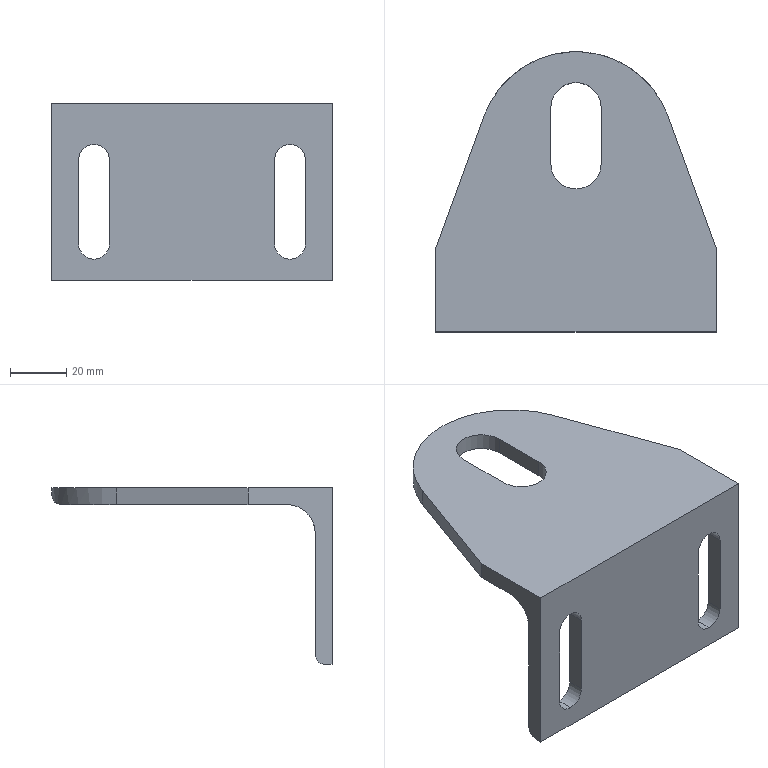Part | SolidWorks | features ICE 2, 3DProfileFeature 1, WeldMemberFeat 1, WeldmentFeature 1 | 1 solid | 29 faces | box 100 x 100 x 63 mm | volume 75285 mm3 | plane 16 | cylinder 13 | commonest cylinder face diameters 11 x6 6.667 x2 18 x2 70 x2 20 x1
STEP:
#1=CARTESIAN_POINT('',(85.,6.,-55.5));
#2=VERTEX_POINT('',#1);
#3=CARTESIAN_POINT('',(90.5,6.,-50.));
#4=VERTEX_POINT('',#3);
#5=CARTESIAN_POINT('',(85.,6.,-50.));
#6=DIRECTION('',(0.,-1.,0.));
#7=DIRECTION('',(0.,0.,-1.));
#8=AXIS2_PLACEMENT_3D('',#5,#6,#7);
#9=CIRCLE('',#8,5.5);
#10=EDGE_CURVE('',#2,#4,#9,.T.);
#11=ORIENTED_EDGE('',*,*,#10,.F.);
#12=CARTESIAN_POINT('',(85.,0.,-55.5));
#13=VERTEX_POINT('',#12);
#14=CARTESIAN_POINT('',(85.,15.,-55.5));
#15=DIRECTION('',(0.,-1.,0.));
#16=VECTOR('',#15,1000.);
#17=LINE('',#14,#16);
#18=EDGE_CURVE('',#2,#13,#17,.T.);
#19=ORIENTED_EDGE('',*,*,#18,.T.);
#20=CARTESIAN_POINT('',(90.5,0.,-50.));
#21=VERTEX_POINT('',#20);
#22=CARTESIAN_POINT('',(85.,0.,-50.));
#23=DIRECTION('',(0.,-1.,0.));
#24=DIRECTION('',(0.,0.,1.));
#25=AXIS2_PLACEMENT_3D('',#22,#23,#24);
#26=CIRCLE('',#25,5.5);
#27=EDGE_CURVE('',#13,#21,#26,.T.);
#28=ORIENTED_EDGE('',*,*,#27,.T.);
#29=CARTESIAN_POINT('',(90.5,15.,-50.));
#30=DIRECTION('',(0.,-1.,0.));
#31=VECTOR('',#30,1000.);
#32=LINE('',#29,#31);
#33=EDGE_CURVE('',#4,#21,#32,.T.);
#34=ORIENTED_EDGE('',*,*,#33,.F.);
#35=EDGE_LOOP('',(#11,#19,#28,#34));
#36=FACE_OUTER_BOUND('',#35,.T.);
#37=CARTESIAN_POINT('',(85.,15.,-50.));
#38=DIRECTION('',(0.,-1.,0.));
#39=DIRECTION('',(0.,0.,-1.));
#40=AXIS2_PLACEMENT_3D('',#37,#38,#39);
#41=CYLINDRICAL_SURFACE('',#40,5.5);
#42=ADVANCED_FACE('',(#36),#41,.F.);
#43=CARTESIAN_POINT('',(15.,6.,-55.5));
#44=VERTEX_POINT('',#43);
#45=CARTESIAN_POINT('',(20.5,6.,-50.));
#46=VERTEX_POINT('',#45);
#47=CARTESIAN_POINT('',(15.,6.,-50.));
#48=DIRECTION('',(0.,-1.,0.));
#49=DIRECTION('',(0.,0.,-1.));
#50=AXIS2_PLACEMENT_3D('',#47,#48,#49);
#51=CIRCLE('',#50,5.5);
#52=EDGE_CURVE('',#44,#46,#51,.T.);
#53=ORIENTED_EDGE('',*,*,#52,.F.);
#54=CARTESIAN_POINT('',(15.,0.,-55.5));
#55=VERTEX_POINT('',#54);
#56=CARTESIAN_POINT('',(15.,15.,-55.5));
#57=DIRECTION('',(0.,-1.,0.));
#58=VECTOR('',#57,1000.);
#59=LINE('',#56,#58);
#60=EDGE_CURVE('',#44,#55,#59,.T.);
#61=ORIENTED_EDGE('',*,*,#60,.T.);
#62=CARTESIAN_POINT('',(20.5,0.,-50.));
#63=VERTEX_POINT('',#62);
#64=CARTESIAN_POINT('',(15.,0.,-50.));
#65=DIRECTION('',(0.,-1.,0.));
#66=DIRECTION('',(0.,0.,-1.));
#67=AXIS2_PLACEMENT_3D('',#64,#65,#66);
#68=CIRCLE('',#67,5.5);
#69=EDGE_CURVE('',#55,#63,#68,.T.);
#70=ORIENTED_EDGE('',*,*,#69,.T.);
#71=CARTESIAN_POINT('',(20.5,15.,-50.));
#72=DIRECTION('',(0.,-1.,0.));
#73=VECTOR('',#72,1000.);
#74=LINE('',#71,#73);
#75=EDGE_CURVE('',#46,#63,#74,.T.);
#76=ORIENTED_EDGE('',*,*,#75,.F.);
#77=EDGE_LOOP('',(#53,#61,#70,#76));
#78=FACE_OUTER_BOUND('',#77,.T.);
#79=CARTESIAN_POINT('',(15.,15.,-50.));
#80=DIRECTION('',(0.,-1.,0.));
#81=DIRECTION('',(0.,0.,-1.));
#82=AXIS2_PLACEMENT_3D('',#79,#80,#81);
#83=CYLINDRICAL_SURFACE('',#82,5.5);
#84=ADVANCED_FACE('',(#78),#83,.F.);
#85=CARTESIAN_POINT('',(59.,60.,-6.));
#86=VERTEX_POINT('',#85);
#87=CARTESIAN_POINT('',(59.,80.,-6.));
#88=VERTEX_POINT('',#87);
#89=CARTESIAN_POINT('',(59.,96.667,-6.));
#90=DIRECTION('',(0.,1.,0.));
#91=VECTOR('',#90,1000.);
#92=LINE('',#89,#91);
#93=EDGE_CURVE('',#86,#88,#92,.T.);
#94=ORIENTED_EDGE('',*,*,#93,.T.);
#95=CARTESIAN_POINT('',(41.,80.,-6.));
#96=VERTEX_POINT('',#95);
#97=CARTESIAN_POINT('',(50.,80.,-6.));
#98=DIRECTION('',(0.,0.,1.));
#99=DIRECTION('',(0.,-1.,0.));
#100=AXIS2_PLACEMENT_3D('',#97,#98,#99);
#101=CIRCLE('',#100,9.);
#102=EDGE_CURVE('',#88,#96,#101,.T.);
#103=ORIENTED_EDGE('',*,*,#102,.T.);
#104=CARTESIAN_POINT('',(41.,60.,-6.));
#105=VERTEX_POINT('',#104);
#106=CARTESIAN_POINT('',(41.,96.667,-6.));
#107=DIRECTION('',(0.,-1.,0.));
#108=VECTOR('',#107,1000.);
#109=LINE('',#106,#108);
#110=EDGE_CURVE('',#96,#105,#109,.T.);
#111=ORIENTED_EDGE('',*,*,#110,.T.);
#112=CARTESIAN_POINT('',(50.,60.,-6.));
#113=DIRECTION('',(0.,0.,1.));
#114=DIRECTION('',(0.,-1.,0.));
#115=AXIS2_PLACEMENT_3D('',#112,#113,#114);
#116=CIRCLE('',#115,9.);
#117=EDGE_CURVE('',#105,#86,#116,.T.);
#118=ORIENTED_EDGE('',*,*,#117,.T.);
#119=EDGE_LOOP('',(#94,#103,#111,#118));
#120=FACE_BOUND('',#119,.T.);
#121=CARTESIAN_POINT('',(17.101,76.985,-6.));
#122=VERTEX_POINT('',#121);
#123=CARTESIAN_POINT('',(0.,30.,-6.));
#124=VERTEX_POINT('',#123);
#125=CARTESIAN_POINT('',(33.124,121.008,-6.));
#126=DIRECTION('',(-0.342,-0.9397,0.));
#127=VECTOR('',#126,1000.);
#128=LINE('',#125,#127);
#129=EDGE_CURVE('',#122,#124,#128,.T.);
#130=ORIENTED_EDGE('',*,*,#129,.F.);
#131=CARTESIAN_POINT('',(35.007,96.667,-6.));
#132=VERTEX_POINT('',#131);
#133=CARTESIAN_POINT('',(50.,65.041,-6.));
#134=DIRECTION('',(0.,0.,1.));
#135=DIRECTION('',(0.,-1.,0.));
#136=AXIS2_PLACEMENT_3D('',#133,#134,#135);
#137=CIRCLE('',#136,35.);
#138=EDGE_CURVE('',#132,#122,#137,.T.);
#139=ORIENTED_EDGE('',*,*,#138,.F.);
#140=CARTESIAN_POINT('',(64.993,96.667,-6.));
#141=VERTEX_POINT('',#140);
#142=CARTESIAN_POINT('',(100.,96.667,-6.));
#143=DIRECTION('',(-1.,0.,0.));
#144=VECTOR('',#143,1000.);
#145=LINE('',#142,#144);
#146=EDGE_CURVE('',#141,#132,#145,.T.);
#147=ORIENTED_EDGE('',*,*,#146,.F.);
#148=CARTESIAN_POINT('',(82.899,76.985,-6.));
#149=VERTEX_POINT('',#148);
#150=CARTESIAN_POINT('',(50.,65.041,-6.));
#151=DIRECTION('',(0.,0.,1.));
#152=DIRECTION('',(0.,-1.,0.));
#153=AXIS2_PLACEMENT_3D('',#150,#151,#152);
#154=CIRCLE('',#153,35.);
#155=EDGE_CURVE('',#149,#141,#154,.T.);
#156=ORIENTED_EDGE('',*,*,#155,.F.);
#157=CARTESIAN_POINT('',(100.,30.,-6.));
#158=VERTEX_POINT('',#157);
#159=CARTESIAN_POINT('',(78.574,88.868,-6.));
#160=DIRECTION('',(-0.342,0.9397,0.));
#161=VECTOR('',#160,1000.);
#162=LINE('',#159,#161);
#163=EDGE_CURVE('',#158,#149,#162,.T.);
#164=ORIENTED_EDGE('',*,*,#163,.F.);
#165=CARTESIAN_POINT('',(100.,16.,-6.));
#166=VERTEX_POINT('',#165);
#167=CARTESIAN_POINT('',(100.,96.667,-6.));
#168=DIRECTION('',(0.,1.,0.));
#169=VECTOR('',#168,1000.);
#170=LINE('',#167,#169);
#171=EDGE_CURVE('',#166,#158,#170,.T.);
#172=ORIENTED_EDGE('',*,*,#171,.F.);
#173=CARTESIAN_POINT('',(0.,16.,-6.));
#174=VERTEX_POINT('',#173);
#175=CARTESIAN_POINT('',(100.,16.,-6.));
#176=DIRECTION('',(-1.,0.,0.));
#177=VECTOR('',#176,1000.);
#178=LINE('',#175,#177);
#179=EDGE_CURVE('',#166,#174,#178,.T.);
#180=ORIENTED_EDGE('',*,*,#179,.T.);
#181=CARTESIAN_POINT('',(0.,96.667,-6.));
#182=DIRECTION('',(0.,1.,0.));
#183=VECTOR('',#182,1000.);
#184=LINE('',#181,#183);
#185=EDGE_CURVE('',#174,#124,#184,.T.);
#186=ORIENTED_EDGE('',*,*,#185,.T.);
#187=EDGE_LOOP('',(#130,#139,#147,#156,#164,#172,#180,#186));
#188=FACE_OUTER_BOUND('',#187,.T.);
#189=CARTESIAN_POINT('',(100.,96.667,-6.));
#190=DIRECTION('',(0.,0.,1.));
#191=DIRECTION('',(0.,-1.,0.));
#192=AXIS2_PLACEMENT_3D('',#189,#190,#191);
#193=PLANE('',#192);
#194=ADVANCED_FACE('',(#120,#188),#193,.F.);
#195=CARTESIAN_POINT('',(51.688,100.,-2.667));
#196=VERTEX_POINT('',#195);
#197=CARTESIAN_POINT('',(64.993,96.667,-6.));
#198=CARTESIAN_POINT('',(63.904,97.183,-6.));
#199=CARTESIAN_POINT('',(62.807,97.635,-5.885));
#200=CARTESIAN_POINT('',(61.142,98.225,-5.621));
#201=CARTESIAN_POINT('',(60.584,98.407,-5.517));
#202=CARTESIAN_POINT('',(59.462,98.743,-5.283));
#203=CARTESIAN_POINT('',(58.896,98.896,-5.152));
#204=CARTESIAN_POINT('',(57.196,99.313,-4.732));
#205=CARTESIAN_POINT('',(56.058,99.532,-4.414));
#206=CARTESIAN_POINT('',(54.353,99.774,-3.889));
#207=CARTESIAN_POINT('',(53.785,99.84,-3.707));
#208=CARTESIAN_POINT('',(52.939,99.918,-3.408));
#209=CARTESIAN_POINT('',(52.658,99.941,-3.304));
#210=CARTESIAN_POINT('',(52.246,99.969,-3.125));
#211=CARTESIAN_POINT('',(52.11,99.977,-3.062));
#212=CARTESIAN_POINT('',(51.916,99.988,-2.948));
#213=CARTESIAN_POINT('',(51.853,99.992,-2.907));
#214=CARTESIAN_POINT('',(51.769,99.996,-2.831));
#215=CARTESIAN_POINT('',(51.743,99.997,-2.804));
#216=CARTESIAN_POINT('',(51.703,99.999,-2.741));
#217=CARTESIAN_POINT('',(51.688,100.,-2.705));
#218=CARTESIAN_POINT('',(51.688,100.,-2.667));
#219=B_SPLINE_CURVE_WITH_KNOTS('',3,(#197,#198,#199,#200,#201,#202,#203,#204,#205,#206,#207,#208,#209,#210,#211,#212,#213,#214,#215,#216,#217,#218),.UNSPECIFIED.,.F.,.F.,(4,2,2,2,2,2,2,2,2,2,4),(0.,0.003571,0.005356,0.007141,0.01071,0.0125,0.01339,0.01384,0.01406,0.01417,0.01428),.UNSPECIFIED.);
#220=EDGE_CURVE('',#141,#196,#219,.T.);
#221=ORIENTED_EDGE('',*,*,#220,.F.);
#222=ORIENTED_EDGE('',*,*,#146,.T.);
#223=CARTESIAN_POINT('',(48.312,100.,-2.667));
#224=VERTEX_POINT('',#223);
#225=CARTESIAN_POINT('',(48.312,100.,-2.667));
#226=CARTESIAN_POINT('',(48.312,100.,-2.705));
#227=CARTESIAN_POINT('',(48.297,99.999,-2.742));
#228=CARTESIAN_POINT('',(48.255,99.997,-2.806));
#229=CARTESIAN_POINT('',(48.229,99.996,-2.834));
#230=CARTESIAN_POINT('',(48.144,99.992,-2.909));
#231=CARTESIAN_POINT('',(48.08,99.988,-2.951));
#232=CARTESIAN_POINT('',(47.885,99.977,-3.065));
#233=CARTESIAN_POINT('',(47.749,99.969,-3.128));
#234=CARTESIAN_POINT('',(47.335,99.94,-3.306));
#235=CARTESIAN_POINT('',(47.053,99.918,-3.41));
#236=CARTESIAN_POINT('',(46.205,99.839,-3.711));
#237=CARTESIAN_POINT('',(45.636,99.772,-3.892));
#238=CARTESIAN_POINT('',(44.497,99.61,-4.243));
#239=CARTESIAN_POINT('',(43.926,99.515,-4.41));
#240=CARTESIAN_POINT('',(42.789,99.295,-4.726));
#241=CARTESIAN_POINT('',(42.223,99.171,-4.876));
#242=CARTESIAN_POINT('',(40.533,98.756,-5.293));
#243=CARTESIAN_POINT('',(39.418,98.423,-5.532));
#244=CARTESIAN_POINT('',(37.203,97.639,-5.884));
#245=CARTESIAN_POINT('',(36.104,97.187,-6.));
#246=CARTESIAN_POINT('',(35.007,96.667,-6.));
#247=B_SPLINE_CURVE_WITH_KNOTS('',3,(#225,#226,#227,#228,#229,#230,#231,#232,#233,#234,#235,#236,#237,#238,#239,#240,#241,#242,#243,#244,#245,#246),.UNSPECIFIED.,.F.,.F.,(4,2,2,2,2,2,2,2,2,2,4),(0.,0.000114,0.000228,0.000456,0.000912,0.001824,0.003648,0.005472,0.007296,0.01094,0.01459),.UNSPECIFIED.);
#248=EDGE_CURVE('',#224,#132,#247,.T.);
#249=ORIENTED_EDGE('',*,*,#248,.F.);
#250=CARTESIAN_POINT('',(100.,100.,-2.667));
#251=DIRECTION('',(-1.,0.,0.));
#252=VECTOR('',#251,1000.);
#253=LINE('',#250,#252);
#254=EDGE_CURVE('',#196,#224,#253,.T.);
#255=ORIENTED_EDGE('',*,*,#254,.F.);
#256=EDGE_LOOP('',(#221,#222,#249,#255));
#257=FACE_OUTER_BOUND('',#256,.T.);
#258=CARTESIAN_POINT('',(100.,96.667,-2.667));
#259=DIRECTION('',(-1.,0.,0.));
#260=DIRECTION('',(0.,0.,1.));
#261=AXIS2_PLACEMENT_3D('',#258,#259,#260);
#262=CYLINDRICAL_SURFACE('',#261,3.333);
#263=ADVANCED_FACE('',(#257),#262,.T.);
#264=CARTESIAN_POINT('',(51.688,100.,0.));
#265=VERTEX_POINT('',#264);
#266=CARTESIAN_POINT('',(51.688,100.,-10.));
#267=DIRECTION('',(0.,0.,1.));
#268=VECTOR('',#267,1000.);
#269=LINE('',#266,#268);
#270=EDGE_CURVE('',#196,#265,#269,.T.);
#271=ORIENTED_EDGE('',*,*,#270,.F.);
#272=ORIENTED_EDGE('',*,*,#254,.T.);
#273=CARTESIAN_POINT('',(48.312,100.,0.));
#274=VERTEX_POINT('',#273);
#275=CARTESIAN_POINT('',(48.312,100.,-10.));
#276=DIRECTION('',(0.,0.,-1.));
#277=VECTOR('',#276,1000.);
#278=LINE('',#275,#277);
#279=EDGE_CURVE('',#274,#224,#278,.T.);
#280=ORIENTED_EDGE('',*,*,#279,.F.);
#281=CARTESIAN_POINT('',(100.,100.,0.));
#282=DIRECTION('',(-1.,0.,0.));
#283=VECTOR('',#282,1000.);
#284=LINE('',#281,#283);
#285=EDGE_CURVE('',#265,#274,#284,.T.);
#286=ORIENTED_EDGE('',*,*,#285,.F.);
#287=EDGE_LOOP('',(#271,#272,#280,#286));
#288=FACE_OUTER_BOUND('',#287,.T.);
#289=CARTESIAN_POINT('',(100.,100.,0.));
#290=DIRECTION('',(0.,-1.,0.));
#291=DIRECTION('',(0.,0.,-1.));
#292=AXIS2_PLACEMENT_3D('',#289,#290,#291);
#293=PLANE('',#292);
#294=ADVANCED_FACE('',(#288),#293,.F.);
#295=CARTESIAN_POINT('',(41.,80.,0.));
#296=VERTEX_POINT('',#295);
#297=CARTESIAN_POINT('',(41.,60.,0.));
#298=VERTEX_POINT('',#297);
#299=CARTESIAN_POINT('',(41.,80.,0.));
#300=DIRECTION('',(0.,-1.,0.));
#301=VECTOR('',#300,1000.);
#302=LINE('',#299,#301);
#303=EDGE_CURVE('',#296,#298,#302,.T.);
#304=ORIENTED_EDGE('',*,*,#303,.F.);
#305=CARTESIAN_POINT('',(59.,80.,0.));
#306=VERTEX_POINT('',#305);
#307=CARTESIAN_POINT('',(50.,80.,0.));
#308=DIRECTION('',(0.,0.,1.));
#309=DIRECTION('',(1.,0.,0.));
#310=AXIS2_PLACEMENT_3D('',#307,#308,#309);
#311=CIRCLE('',#310,9.);
#312=EDGE_CURVE('',#306,#296,#311,.T.);
#313=ORIENTED_EDGE('',*,*,#312,.F.);
#314=CARTESIAN_POINT('',(59.,60.,0.));
#315=VERTEX_POINT('',#314);
#316=CARTESIAN_POINT('',(59.,80.,0.));
#317=DIRECTION('',(0.,1.,0.));
#318=VECTOR('',#317,1000.);
#319=LINE('',#316,#318);
#320=EDGE_CURVE('',#315,#306,#319,.T.);
#321=ORIENTED_EDGE('',*,*,#320,.F.);
#322=CARTESIAN_POINT('',(50.,60.,0.));
#323=DIRECTION('',(0.,0.,1.));
#324=DIRECTION('',(1.,0.,0.));
#325=AXIS2_PLACEMENT_3D('',#322,#323,#324);
#326=CIRCLE('',#325,9.);
#327=EDGE_CURVE('',#298,#315,#326,.T.);
#328=ORIENTED_EDGE('',*,*,#327,.F.);
#329=EDGE_LOOP('',(#304,#313,#321,#328));
#330=FACE_BOUND('',#329,.T.);
#331=CARTESIAN_POINT('',(17.101,76.985,0.));
#332=VERTEX_POINT('',#331);
#333=CARTESIAN_POINT('',(0.,30.,0.));
#334=VERTEX_POINT('',#333);
#335=CARTESIAN_POINT('',(0.,30.,0.));
#336=DIRECTION('',(-0.342,-0.9397,0.));
#337=VECTOR('',#336,1000.);
#338=LINE('',#335,#337);
#339=EDGE_CURVE('',#332,#334,#338,.T.);
#340=ORIENTED_EDGE('',*,*,#339,.T.);
#341=CARTESIAN_POINT('',(0.,0.,0.));
#342=VERTEX_POINT('',#341);
#343=CARTESIAN_POINT('',(0.,0.,0.));
#344=DIRECTION('',(0.,-1.,0.));
#345=VECTOR('',#344,1000.);
#346=LINE('',#343,#345);
#347=EDGE_CURVE('',#334,#342,#346,.T.);
#348=ORIENTED_EDGE('',*,*,#347,.T.);
#349=CARTESIAN_POINT('',(100.,0.,0.));
#350=VERTEX_POINT('',#349);
#351=CARTESIAN_POINT('',(100.,0.,0.));
#352=DIRECTION('',(-1.,0.,0.));
#353=VECTOR('',#352,1000.);
#354=LINE('',#351,#353);
#355=EDGE_CURVE('',#350,#342,#354,.T.);
#356=ORIENTED_EDGE('',*,*,#355,.F.);
#357=CARTESIAN_POINT('',(100.,30.,0.));
#358=VERTEX_POINT('',#357);
#359=CARTESIAN_POINT('',(100.,0.,0.));
#360=DIRECTION('',(0.,-1.,0.));
#361=VECTOR('',#360,1000.);
#362=LINE('',#359,#361);
#363=EDGE_CURVE('',#358,#350,#362,.T.);
#364=ORIENTED_EDGE('',*,*,#363,.F.);
#365=CARTESIAN_POINT('',(82.899,76.985,0.));
#366=VERTEX_POINT('',#365);
#367=CARTESIAN_POINT('',(100.,30.,0.));
#368=DIRECTION('',(-0.342,0.9397,0.));
#369=VECTOR('',#368,1000.);
#370=LINE('',#367,#369);
#371=EDGE_CURVE('',#358,#366,#370,.T.);
#372=ORIENTED_EDGE('',*,*,#371,.T.);
#373=CARTESIAN_POINT('',(50.,65.041,0.));
#374=DIRECTION('',(0.,0.,1.));
#375=DIRECTION('',(-1.,0.,0.));
#376=AXIS2_PLACEMENT_3D('',#373,#374,#375);
#377=CIRCLE('',#376,35.);
#378=EDGE_CURVE('',#366,#265,#377,.T.);
#379=ORIENTED_EDGE('',*,*,#378,.T.);
#380=ORIENTED_EDGE('',*,*,#285,.T.);
#381=CARTESIAN_POINT('',(50.,65.041,0.));
#382=DIRECTION('',(0.,0.,1.));
#383=DIRECTION('',(-1.,0.,0.));
#384=AXIS2_PLACEMENT_3D('',#381,#382,#383);
#385=CIRCLE('',#384,35.);
#386=EDGE_CURVE('',#274,#332,#385,.T.);
#387=ORIENTED_EDGE('',*,*,#386,.T.);
#388=EDGE_LOOP('',(#340,#348,#356,#364,#372,#379,#380,#387));
#389=FACE_OUTER_BOUND('',#388,.T.);
#390=CARTESIAN_POINT('',(100.,0.,0.));
#391=DIRECTION('',(0.,0.,-1.));
#392=DIRECTION('',(-1.,0.,0.));
#393=AXIS2_PLACEMENT_3D('',#390,#391,#392);
#394=PLANE('',#393);
#395=ADVANCED_FACE('',(#330,#389),#394,.F.);
#396=CARTESIAN_POINT('',(100.,0.,-63.));
#397=VERTEX_POINT('',#396);
#398=CARTESIAN_POINT('',(100.,0.,-63.));
#399=DIRECTION('',(0.,0.,-1.));
#400=VECTOR('',#399,1000.);
#401=LINE('',#398,#400);
#402=EDGE_CURVE('',#350,#397,#401,.T.);
#403=ORIENTED_EDGE('',*,*,#402,.T.);
#404=CARTESIAN_POINT('',(100.,2.667,-63.));
#405=VERTEX_POINT('',#404);
#406=CARTESIAN_POINT('',(100.,0.,-63.));
#407=DIRECTION('',(0.,1.,0.));
#408=VECTOR('',#407,1000.);
#409=LINE('',#406,#408);
#410=EDGE_CURVE('',#397,#405,#409,.T.);
#411=ORIENTED_EDGE('',*,*,#410,.T.);
#412=CARTESIAN_POINT('',(100.,6.,-59.667));
#413=VERTEX_POINT('',#412);
#414=CARTESIAN_POINT('',(100.,2.667,-59.667));
#415=DIRECTION('',(1.,0.,0.));
#416=DIRECTION('',(0.,0.,-1.));
#417=AXIS2_PLACEMENT_3D('',#414,#415,#416);
#418=CIRCLE('',#417,3.333);
#419=EDGE_CURVE('',#405,#413,#418,.T.);
#420=ORIENTED_EDGE('',*,*,#419,.T.);
#421=CARTESIAN_POINT('',(100.,6.,-16.));
#422=VERTEX_POINT('',#421);
#423=CARTESIAN_POINT('',(100.,6.,-16.));
#424=DIRECTION('',(0.,0.,1.));
#425=VECTOR('',#424,1000.);
#426=LINE('',#423,#425);
#427=EDGE_CURVE('',#413,#422,#426,.T.);
#428=ORIENTED_EDGE('',*,*,#427,.T.);
#429=CARTESIAN_POINT('',(100.,16.,-16.));
#430=DIRECTION('',(-1.,0.,0.));
#431=DIRECTION('',(0.,0.,1.));
#432=AXIS2_PLACEMENT_3D('',#429,#430,#431);
#433=CIRCLE('',#432,10.);
#434=EDGE_CURVE('',#422,#166,#433,.T.);
#435=ORIENTED_EDGE('',*,*,#434,.T.);
#436=ORIENTED_EDGE('',*,*,#171,.T.);
#437=CARTESIAN_POINT('',(100.,30.,-2.667));
#438=DIRECTION('',(0.,0.,-1.));
#439=VECTOR('',#438,1000.);
#440=LINE('',#437,#439);
#441=EDGE_CURVE('',#358,#158,#440,.T.);
#442=ORIENTED_EDGE('',*,*,#441,.F.);
#443=ORIENTED_EDGE('',*,*,#363,.T.);
#444=EDGE_LOOP('',(#403,#411,#420,#428,#435,#436,#442,#443));
#445=FACE_OUTER_BOUND('',#444,.T.);
#446=CARTESIAN_POINT('',(100.,96.667,-2.667));
#447=DIRECTION('',(-1.,0.,0.));
#448=DIRECTION('',(0.,0.,1.));
#449=AXIS2_PLACEMENT_3D('',#446,#447,#448);
#450=PLANE('',#449);
#451=ADVANCED_FACE('',(#445),#450,.F.);
#452=ORIENTED_EDGE('',*,*,#185,.F.);
#453=CARTESIAN_POINT('',(0.,6.,-16.));
#454=VERTEX_POINT('',#453);
#455=CARTESIAN_POINT('',(0.,16.,-16.));
#456=DIRECTION('',(-1.,0.,0.));
#457=DIRECTION('',(0.,0.,1.));
#458=AXIS2_PLACEMENT_3D('',#455,#456,#457);
#459=CIRCLE('',#458,10.);
#460=EDGE_CURVE('',#454,#174,#459,.T.);
#461=ORIENTED_EDGE('',*,*,#460,.F.);
#462=CARTESIAN_POINT('',(0.,6.,-59.667));
#463=VERTEX_POINT('',#462);
#464=CARTESIAN_POINT('',(0.,6.,-16.));
#465=DIRECTION('',(0.,0.,1.));
#466=VECTOR('',#465,1000.);
#467=LINE('',#464,#466);
#468=EDGE_CURVE('',#463,#454,#467,.T.);
#469=ORIENTED_EDGE('',*,*,#468,.F.);
#470=CARTESIAN_POINT('',(0.,2.667,-63.));
#471=VERTEX_POINT('',#470);
#472=CARTESIAN_POINT('',(0.,2.667,-59.667));
#473=DIRECTION('',(1.,0.,0.));
#474=DIRECTION('',(0.,0.,-1.));
#475=AXIS2_PLACEMENT_3D('',#472,#473,#474);
#476=CIRCLE('',#475,3.333);
#477=EDGE_CURVE('',#471,#463,#476,.T.);
#478=ORIENTED_EDGE('',*,*,#477,.F.);
#479=CARTESIAN_POINT('',(0.,0.,-63.));
#480=VERTEX_POINT('',#479);
#481=CARTESIAN_POINT('',(0.,0.,-63.));
#482=DIRECTION('',(0.,1.,0.));
#483=VECTOR('',#482,1000.);
#484=LINE('',#481,#483);
#485=EDGE_CURVE('',#480,#471,#484,.T.);
#486=ORIENTED_EDGE('',*,*,#485,.F.);
#487=CARTESIAN_POINT('',(0.,0.,-63.));
#488=DIRECTION('',(0.,0.,-1.));
#489=VECTOR('',#488,1000.);
#490=LINE('',#487,#489);
#491=EDGE_CURVE('',#342,#480,#490,.T.);
#492=ORIENTED_EDGE('',*,*,#491,.F.);
#493=ORIENTED_EDGE('',*,*,#347,.F.);
#494=CARTESIAN_POINT('',(0.,30.,-2.667));
#495=DIRECTION('',(0.,0.,-1.));
#496=VECTOR('',#495,1000.);
#497=LINE('',#494,#496);
#498=EDGE_CURVE('',#334,#124,#497,.T.);
#499=ORIENTED_EDGE('',*,*,#498,.T.);
#500=EDGE_LOOP('',(#452,#461,#469,#478,#486,#492,#493,#499));
#501=FACE_OUTER_BOUND('',#500,.T.);
#502=CARTESIAN_POINT('',(0.,96.667,-2.667));
#503=DIRECTION('',(-1.,0.,0.));
#504=DIRECTION('',(0.,0.,1.));
#505=AXIS2_PLACEMENT_3D('',#502,#503,#504);
#506=PLANE('',#505);
#507=ADVANCED_FACE('',(#501),#506,.T.);
#508=CARTESIAN_POINT('',(79.5,0.,-20.));
#509=VERTEX_POINT('',#508);
#510=CARTESIAN_POINT('',(79.5,0.,-50.));
#511=VERTEX_POINT('',#510);
#512=CARTESIAN_POINT('',(79.5,0.,-20.));
#513=DIRECTION('',(0.,0.,-1.));
#514=VECTOR('',#513,1000.);
#515=LINE('',#512,#514);
#516=EDGE_CURVE('',#509,#511,#515,.T.);
#517=ORIENTED_EDGE('',*,*,#516,.F.);
#518=CARTESIAN_POINT('',(90.5,0.,-20.));
#519=VERTEX_POINT('',#518);
#520=CARTESIAN_POINT('',(85.,0.,-20.));
#521=DIRECTION('',(0.,-1.,0.));
#522=DIRECTION('',(0.,0.,1.));
#523=AXIS2_PLACEMENT_3D('',#520,#521,#522);
#524=CIRCLE('',#523,5.5);
#525=EDGE_CURVE('',#519,#509,#524,.T.);
#526=ORIENTED_EDGE('',*,*,#525,.F.);
#527=CARTESIAN_POINT('',(90.5,0.,-20.));
#528=DIRECTION('',(0.,0.,1.));
#529=VECTOR('',#528,1000.);
#530=LINE('',#527,#529);
#531=EDGE_CURVE('',#21,#519,#530,.T.);
#532=ORIENTED_EDGE('',*,*,#531,.F.);
#533=ORIENTED_EDGE('',*,*,#27,.F.);
#534=CARTESIAN_POINT('',(85.,0.,-50.));
#535=DIRECTION('',(0.,-1.,0.));
#536=DIRECTION('',(0.,0.,1.));
#537=AXIS2_PLACEMENT_3D('',#534,#535,#536);
#538=CIRCLE('',#537,5.5);
#539=EDGE_CURVE('',#511,#13,#538,.T.);
#540=ORIENTED_EDGE('',*,*,#539,.F.);
#541=EDGE_LOOP('',(#517,#526,#532,#533,#540));
#542=FACE_BOUND('',#541,.T.);
#543=CARTESIAN_POINT('',(9.5,0.,-20.));
#544=VERTEX_POINT('',#543);
#545=CARTESIAN_POINT('',(9.5,0.,-50.));
#546=VERTEX_POINT('',#545);
#547=CARTESIAN_POINT('',(9.5,0.,-20.));
#548=DIRECTION('',(0.,0.,-1.));
#549=VECTOR('',#548,1000.);
#550=LINE('',#547,#549);
#551=EDGE_CURVE('',#544,#546,#550,.T.);
#552=ORIENTED_EDGE('',*,*,#551,.F.);
#553=CARTESIAN_POINT('',(20.5,0.,-20.));
#554=VERTEX_POINT('',#553);
#555=CARTESIAN_POINT('',(15.,0.,-20.));
#556=DIRECTION('',(0.,-1.,0.));
#557=DIRECTION('',(0.,0.,-1.));
#558=AXIS2_PLACEMENT_3D('',#555,#556,#557);
#559=CIRCLE('',#558,5.5);
#560=EDGE_CURVE('',#554,#544,#559,.T.);
#561=ORIENTED_EDGE('',*,*,#560,.F.);
#562=CARTESIAN_POINT('',(20.5,0.,-20.));
#563=DIRECTION('',(0.,0.,1.));
#564=VECTOR('',#563,1000.);
#565=LINE('',#562,#564);
#566=EDGE_CURVE('',#63,#554,#565,.T.);
#567=ORIENTED_EDGE('',*,*,#566,.F.);
#568=ORIENTED_EDGE('',*,*,#69,.F.);
#569=CARTESIAN_POINT('',(15.,0.,-50.));
#570=DIRECTION('',(0.,-1.,0.));
#571=DIRECTION('',(0.,0.,-1.));
#572=AXIS2_PLACEMENT_3D('',#569,#570,#571);
#573=CIRCLE('',#572,5.5);
#574=EDGE_CURVE('',#546,#55,#573,.T.);
#575=ORIENTED_EDGE('',*,*,#574,.F.);
#576=EDGE_LOOP('',(#552,#561,#567,#568,#575));
#577=FACE_BOUND('',#576,.T.);
#578=ORIENTED_EDGE('',*,*,#491,.T.);
#579=CARTESIAN_POINT('',(100.,0.,-63.));
#580=DIRECTION('',(-1.,0.,0.));
#581=VECTOR('',#580,1000.);
#582=LINE('',#579,#581);
#583=EDGE_CURVE('',#397,#480,#582,.T.);
#584=ORIENTED_EDGE('',*,*,#583,.F.);
#585=ORIENTED_EDGE('',*,*,#402,.F.);
#586=ORIENTED_EDGE('',*,*,#355,.T.);
#587=EDGE_LOOP('',(#578,#584,#585,#586));
#588=FACE_OUTER_BOUND('',#587,.T.);
#589=CARTESIAN_POINT('',(100.,0.,-63.));
#590=DIRECTION('',(0.,1.,0.));
#591=DIRECTION('',(0.,0.,1.));
#592=AXIS2_PLACEMENT_3D('',#589,#590,#591);
#593=PLANE('',#592);
#594=ADVANCED_FACE('',(#542,#577,#588),#593,.F.);
#595=ORIENTED_EDGE('',*,*,#485,.T.);
#596=CARTESIAN_POINT('',(100.,2.667,-63.));
#597=DIRECTION('',(-1.,0.,0.));
#598=VECTOR('',#597,1000.);
#599=LINE('',#596,#598);
#600=EDGE_CURVE('',#405,#471,#599,.T.);
#601=ORIENTED_EDGE('',*,*,#600,.F.);
#602=ORIENTED_EDGE('',*,*,#410,.F.);
#603=ORIENTED_EDGE('',*,*,#583,.T.);
#604=EDGE_LOOP('',(#595,#601,#602,#603));
#605=FACE_OUTER_BOUND('',#604,.T.);
#606=CARTESIAN_POINT('',(100.,0.,-63.));
#607=DIRECTION('',(0.,0.,1.));
#608=DIRECTION('',(1.,0.,0.));
#609=AXIS2_PLACEMENT_3D('',#606,#607,#608);
#610=PLANE('',#609);
#611=ADVANCED_FACE('',(#605),#610,.F.);
#612=ORIENTED_EDGE('',*,*,#477,.T.);
#613=CARTESIAN_POINT('',(100.,6.,-59.667));
#614=DIRECTION('',(-1.,0.,0.));
#615=VECTOR('',#614,1000.);
#616=LINE('',#613,#615);
#617=EDGE_CURVE('',#413,#463,#616,.T.);
#618=ORIENTED_EDGE('',*,*,#617,.F.);
#619=ORIENTED_EDGE('',*,*,#419,.F.);
#620=ORIENTED_EDGE('',*,*,#600,.T.);
#621=EDGE_LOOP('',(#612,#618,#619,#620));
#622=FACE_OUTER_BOUND('',#621,.T.);
#623=CARTESIAN_POINT('',(100.,2.667,-59.667));
#624=DIRECTION('',(-1.,0.,0.));
#625=DIRECTION('',(0.,0.,1.));
#626=AXIS2_PLACEMENT_3D('',#623,#624,#625);
#627=CYLINDRICAL_SURFACE('',#626,3.333);
#628=ADVANCED_FACE('',(#622),#627,.T.);
#629=CARTESIAN_POINT('',(90.5,6.,-20.));
#630=VERTEX_POINT('',#629);
#631=CARTESIAN_POINT('',(90.5,6.,-16.));
#632=DIRECTION('',(0.,0.,1.));
#633=VECTOR('',#632,1000.);
#634=LINE('',#631,#633);
#635=EDGE_CURVE('',#4,#630,#634,.T.);
#636=ORIENTED_EDGE('',*,*,#635,.T.);
#637=CARTESIAN_POINT('',(88.775,6.,-16.));
#638=VERTEX_POINT('',#637);
#639=CARTESIAN_POINT('',(85.,6.,-20.));
#640=DIRECTION('',(0.,-1.,0.));
#641=DIRECTION('',(0.,0.,-1.));
#642=AXIS2_PLACEMENT_3D('',#639,#640,#641);
#643=CIRCLE('',#642,5.5);
#644=EDGE_CURVE('',#630,#638,#643,.T.);
#645=ORIENTED_EDGE('',*,*,#644,.T.);
#646=CARTESIAN_POINT('',(100.,6.,-16.));
#647=DIRECTION('',(-1.,0.,0.));
#648=VECTOR('',#647,1000.);
#649=LINE('',#646,#648);
#650=EDGE_CURVE('',#422,#638,#649,.T.);
#651=ORIENTED_EDGE('',*,*,#650,.F.);
#652=ORIENTED_EDGE('',*,*,#427,.F.);
#653=ORIENTED_EDGE('',*,*,#617,.T.);
#654=ORIENTED_EDGE('',*,*,#468,.T.);
#655=CARTESIAN_POINT('',(11.225,6.,-16.));
#656=VERTEX_POINT('',#655);
#657=CARTESIAN_POINT('',(100.,6.,-16.));
#658=DIRECTION('',(-1.,0.,0.));
#659=VECTOR('',#658,1000.);
#660=LINE('',#657,#659);
#661=EDGE_CURVE('',#656,#454,#660,.T.);
#662=ORIENTED_EDGE('',*,*,#661,.F.);
#663=CARTESIAN_POINT('',(9.5,6.,-20.));
#664=VERTEX_POINT('',#663);
#665=CARTESIAN_POINT('',(15.,6.,-20.));
#666=DIRECTION('',(0.,-1.,0.));
#667=DIRECTION('',(0.,0.,-1.));
#668=AXIS2_PLACEMENT_3D('',#665,#666,#667);
#669=CIRCLE('',#668,5.5);
#670=EDGE_CURVE('',#656,#664,#669,.T.);
#671=ORIENTED_EDGE('',*,*,#670,.T.);
#672=CARTESIAN_POINT('',(9.5,6.,-50.));
#673=VERTEX_POINT('',#672);
#674=CARTESIAN_POINT('',(9.5,6.,-16.));
#675=DIRECTION('',(0.,0.,-1.));
#676=VECTOR('',#675,1000.);
#677=LINE('',#674,#676);
#678=EDGE_CURVE('',#664,#673,#677,.T.);
#679=ORIENTED_EDGE('',*,*,#678,.T.);
#680=CARTESIAN_POINT('',(15.,6.,-50.));
#681=DIRECTION('',(0.,-1.,0.));
#682=DIRECTION('',(0.,0.,-1.));
#683=AXIS2_PLACEMENT_3D('',#680,#681,#682);
#684=CIRCLE('',#683,5.5);
#685=EDGE_CURVE('',#673,#44,#684,.T.);
#686=ORIENTED_EDGE('',*,*,#685,.T.);
#687=ORIENTED_EDGE('',*,*,#52,.T.);
#688=CARTESIAN_POINT('',(20.5,6.,-20.));
#689=VERTEX_POINT('',#688);
#690=CARTESIAN_POINT('',(20.5,6.,-16.));
#691=DIRECTION('',(0.,0.,1.));
#692=VECTOR('',#691,1000.);
#693=LINE('',#690,#692);
#694=EDGE_CURVE('',#46,#689,#693,.T.);
#695=ORIENTED_EDGE('',*,*,#694,.T.);
#696=CARTESIAN_POINT('',(18.775,6.,-16.));
#697=VERTEX_POINT('',#696);
#698=CARTESIAN_POINT('',(15.,6.,-20.));
#699=DIRECTION('',(0.,-1.,0.));
#700=DIRECTION('',(0.,0.,-1.));
#701=AXIS2_PLACEMENT_3D('',#698,#699,#700);
#702=CIRCLE('',#701,5.5);
#703=EDGE_CURVE('',#689,#697,#702,.T.);
#704=ORIENTED_EDGE('',*,*,#703,.T.);
#705=CARTESIAN_POINT('',(81.225,6.,-16.));
#706=VERTEX_POINT('',#705);
#707=CARTESIAN_POINT('',(100.,6.,-16.));
#708=DIRECTION('',(-1.,0.,0.));
#709=VECTOR('',#708,1000.);
#710=LINE('',#707,#709);
#711=EDGE_CURVE('',#706,#697,#710,.T.);
#712=ORIENTED_EDGE('',*,*,#711,.F.);
#713=CARTESIAN_POINT('',(79.5,6.,-20.));
#714=VERTEX_POINT('',#713);
#715=CARTESIAN_POINT('',(85.,6.,-20.));
#716=DIRECTION('',(0.,-1.,0.));
#717=DIRECTION('',(0.,0.,-1.));
#718=AXIS2_PLACEMENT_3D('',#715,#716,#717);
#719=CIRCLE('',#718,5.5);
#720=EDGE_CURVE('',#706,#714,#719,.T.);
#721=ORIENTED_EDGE('',*,*,#720,.T.);
#722=CARTESIAN_POINT('',(79.5,6.,-50.));
#723=VERTEX_POINT('',#722);
#724=CARTESIAN_POINT('',(79.5,6.,-16.));
#725=DIRECTION('',(0.,0.,-1.));
#726=VECTOR('',#725,1000.);
#727=LINE('',#724,#726);
#728=EDGE_CURVE('',#714,#723,#727,.T.);
#729=ORIENTED_EDGE('',*,*,#728,.T.);
#730=CARTESIAN_POINT('',(85.,6.,-50.));
#731=DIRECTION('',(0.,-1.,0.));
#732=DIRECTION('',(0.,0.,-1.));
#733=AXIS2_PLACEMENT_3D('',#730,#731,#732);
#734=CIRCLE('',#733,5.5);
#735=EDGE_CURVE('',#723,#2,#734,.T.);
#736=ORIENTED_EDGE('',*,*,#735,.T.);
#737=ORIENTED_EDGE('',*,*,#10,.T.);
#738=EDGE_LOOP('',(#636,#645,#651,#652,#653,#654,#662,#671,#679,#686,#687,#695,#704,#712,#721,#729,#736,#737));
#739=FACE_OUTER_BOUND('',#738,.T.);
#740=CARTESIAN_POINT('',(100.,6.,-16.));
#741=DIRECTION('',(0.,-1.,0.));
#742=DIRECTION('',(0.,0.,-1.));
#743=AXIS2_PLACEMENT_3D('',#740,#741,#742);
#744=PLANE('',#743);
#745=ADVANCED_FACE('',(#739),#744,.F.);
#746=ORIENTED_EDGE('',*,*,#650,.T.);
#747=CARTESIAN_POINT('',(88.775,6.,-16.));
#748=CARTESIAN_POINT('',(88.523,6.,-15.762));
#749=CARTESIAN_POINT('',(88.245,6.009,-15.546));
#750=CARTESIAN_POINT('',(87.661,6.032,-15.174));
#751=CARTESIAN_POINT('',(87.354,6.048,-15.017));
#752=CARTESIAN_POINT('',(86.869,6.069,-14.824));
#753=CARTESIAN_POINT('',(86.703,6.076,-14.767));
#754=CARTESIAN_POINT('',(86.37,6.089,-14.67));
#755=CARTESIAN_POINT('',(86.202,6.094,-14.63));
#756=CARTESIAN_POINT('',(85.694,6.108,-14.533));
#757=CARTESIAN_POINT('',(85.349,6.113,-14.5));
#758=CARTESIAN_POINT('',(84.649,6.113,-14.5));
#759=CARTESIAN_POINT('',(84.305,6.108,-14.533));
#760=CARTESIAN_POINT('',(83.797,6.094,-14.63));
#761=CARTESIAN_POINT('',(83.629,6.089,-14.671));
#762=CARTESIAN_POINT('',(83.295,6.076,-14.768));
#763=CARTESIAN_POINT('',(83.129,6.069,-14.825));
#764=CARTESIAN_POINT('',(82.645,6.048,-15.018));
#765=CARTESIAN_POINT('',(82.338,6.032,-15.175));
#766=CARTESIAN_POINT('',(81.755,6.009,-15.546));
#767=CARTESIAN_POINT('',(81.477,6.,-15.763));
#768=CARTESIAN_POINT('',(81.225,6.,-16.));
#769=B_SPLINE_CURVE_WITH_KNOTS('',3,(#747,#748,#749,#750,#751,#752,#753,#754,#755,#756,#757,#758,#759,#760,#761,#762,#763,#764,#765,#766,#767,#768),.UNSPECIFIED.,.F.,.F.,(4,2,2,2,2,2,2,2,2,2,4),(0.004571,0.005607,0.006643,0.007161,0.007679,0.008715,0.009751,0.01027,0.01079,0.01182,0.01286),.UNSPECIFIED.);
#770=EDGE_CURVE('',#638,#706,#769,.T.);
#771=ORIENTED_EDGE('',*,*,#770,.T.);
#772=ORIENTED_EDGE('',*,*,#711,.T.);
#773=CARTESIAN_POINT('',(18.775,6.,-16.));
#774=CARTESIAN_POINT('',(18.52,6.,-15.76));
#775=CARTESIAN_POINT('',(18.247,6.009,-15.548));
#776=CARTESIAN_POINT('',(17.811,6.026,-15.27));
#777=CARTESIAN_POINT('',(17.661,6.033,-15.184));
#778=CARTESIAN_POINT('',(17.353,6.047,-15.026));
#779=CARTESIAN_POINT('',(17.193,6.055,-14.953));
#780=CARTESIAN_POINT('',(16.709,6.076,-14.761));
#781=CARTESIAN_POINT('',(16.377,6.089,-14.664));
#782=CARTESIAN_POINT('',(15.699,6.108,-14.534));
#783=CARTESIAN_POINT('',(15.348,6.113,-14.5));
#784=CARTESIAN_POINT('',(14.656,6.113,-14.5));
#785=CARTESIAN_POINT('',(14.312,6.108,-14.532));
#786=CARTESIAN_POINT('',(13.631,6.09,-14.662));
#787=CARTESIAN_POINT('',(13.293,6.076,-14.76));
#788=CARTESIAN_POINT('',(12.652,6.048,-15.014));
#789=CARTESIAN_POINT('',(12.344,6.033,-15.171));
#790=CARTESIAN_POINT('',(11.756,6.009,-15.545));
#791=CARTESIAN_POINT('',(11.48,6.,-15.76));
#792=CARTESIAN_POINT('',(11.225,6.,-16.));
#793=B_SPLINE_CURVE_WITH_KNOTS('',3,(#773,#774,#775,#776,#777,#778,#779,#780,#781,#782,#783,#784,#785,#786,#787,#788,#789,#790,#791,#792),.UNSPECIFIED.,.F.,.F.,(4,2,2,2,2,2,2,2,2,4),(0.,0.001035,0.001552,0.00207,0.003104,0.004139,0.005174,0.006209,0.007243,0.008278),.UNSPECIFIED.);
#794=EDGE_CURVE('',#697,#656,#793,.T.);
#795=ORIENTED_EDGE('',*,*,#794,.T.);
#796=ORIENTED_EDGE('',*,*,#661,.T.);
#797=ORIENTED_EDGE('',*,*,#460,.T.);
#798=ORIENTED_EDGE('',*,*,#179,.F.);
#799=ORIENTED_EDGE('',*,*,#434,.F.);
#800=EDGE_LOOP('',(#746,#771,#772,#795,#796,#797,#798,#799));
#801=FACE_OUTER_BOUND('',#800,.T.);
#802=CARTESIAN_POINT('',(100.,16.,-16.));
#803=DIRECTION('',(-1.,0.,0.));
#804=DIRECTION('',(0.,0.,1.));
#805=AXIS2_PLACEMENT_3D('',#802,#803,#804);
#806=CYLINDRICAL_SURFACE('',#805,10.);
#807=ADVANCED_FACE('',(#801),#806,.F.);
#808=CARTESIAN_POINT('',(59.,80.,-10.));
#809=DIRECTION('',(0.,0.,1.));
#810=VECTOR('',#809,1000.);
#811=LINE('',#808,#810);
#812=EDGE_CURVE('',#88,#306,#811,.T.);
#813=ORIENTED_EDGE('',*,*,#812,.T.);
#814=ORIENTED_EDGE('',*,*,#312,.T.);
#815=CARTESIAN_POINT('',(41.,80.,-10.));
#816=DIRECTION('',(0.,0.,1.));
#817=VECTOR('',#816,1000.);
#818=LINE('',#815,#817);
#819=EDGE_CURVE('',#96,#296,#818,.T.);
#820=ORIENTED_EDGE('',*,*,#819,.F.);
#821=ORIENTED_EDGE('',*,*,#102,.F.);
#822=EDGE_LOOP('',(#813,#814,#820,#821));
#823=FACE_OUTER_BOUND('',#822,.T.);
#824=CARTESIAN_POINT('',(50.,80.,-10.));
#825=DIRECTION('',(0.,0.,1.));
#826=DIRECTION('',(1.,0.,0.));
#827=AXIS2_PLACEMENT_3D('',#824,#825,#826);
#828=CYLINDRICAL_SURFACE('',#827,9.);
#829=ADVANCED_FACE('',(#823),#828,.F.);
#830=CARTESIAN_POINT('',(59.,60.,-10.));
#831=DIRECTION('',(0.,0.,1.));
#832=VECTOR('',#831,1000.);
#833=LINE('',#830,#832);
#834=EDGE_CURVE('',#86,#315,#833,.T.);
#835=ORIENTED_EDGE('',*,*,#834,.T.);
#836=ORIENTED_EDGE('',*,*,#320,.T.);
#837=ORIENTED_EDGE('',*,*,#812,.F.);
#838=ORIENTED_EDGE('',*,*,#93,.F.);
#839=EDGE_LOOP('',(#835,#836,#837,#838));
#840=FACE_OUTER_BOUND('',#839,.T.);
#841=CARTESIAN_POINT('',(59.,80.,-10.));
#842=DIRECTION('',(1.,0.,0.));
#843=DIRECTION('',(0.,0.,-1.));
#844=AXIS2_PLACEMENT_3D('',#841,#842,#843);
#845=PLANE('',#844);
#846=ADVANCED_FACE('',(#840),#845,.F.);
#847=CARTESIAN_POINT('',(41.,60.,-10.));
#848=DIRECTION('',(0.,0.,1.));
#849=VECTOR('',#848,1000.);
#850=LINE('',#847,#849);
#851=EDGE_CURVE('',#105,#298,#850,.T.);
#852=ORIENTED_EDGE('',*,*,#851,.T.);
#853=ORIENTED_EDGE('',*,*,#327,.T.);
#854=ORIENTED_EDGE('',*,*,#834,.F.);
#855=ORIENTED_EDGE('',*,*,#117,.F.);
#856=EDGE_LOOP('',(#852,#853,#854,#855));
#857=FACE_OUTER_BOUND('',#856,.T.);
#858=CARTESIAN_POINT('',(50.,60.,-10.));
#859=DIRECTION('',(0.,0.,1.));
#860=DIRECTION('',(1.,0.,0.));
#861=AXIS2_PLACEMENT_3D('',#858,#859,#860);
#862=CYLINDRICAL_SURFACE('',#861,9.);
#863=ADVANCED_FACE('',(#857),#862,.F.);
#864=ORIENTED_EDGE('',*,*,#819,.T.);
#865=ORIENTED_EDGE('',*,*,#303,.T.);
#866=ORIENTED_EDGE('',*,*,#851,.F.);
#867=ORIENTED_EDGE('',*,*,#110,.F.);
#868=EDGE_LOOP('',(#864,#865,#866,#867));
#869=FACE_OUTER_BOUND('',#868,.T.);
#870=CARTESIAN_POINT('',(41.,80.,-10.));
#871=DIRECTION('',(-1.,0.,0.));
#872=DIRECTION('',(0.,0.,1.));
#873=AXIS2_PLACEMENT_3D('',#870,#871,#872);
#874=PLANE('',#873);
#875=ADVANCED_FACE('',(#869),#874,.F.);
#876=ORIENTED_EDGE('',*,*,#129,.T.);
#877=ORIENTED_EDGE('',*,*,#498,.F.);
#878=ORIENTED_EDGE('',*,*,#339,.F.);
#879=CARTESIAN_POINT('',(17.101,76.985,-10.));
#880=DIRECTION('',(0.,0.,1.));
#881=VECTOR('',#880,1000.);
#882=LINE('',#879,#881);
#883=EDGE_CURVE('',#122,#332,#882,.T.);
#884=ORIENTED_EDGE('',*,*,#883,.F.);
#885=EDGE_LOOP('',(#876,#877,#878,#884));
#886=FACE_OUTER_BOUND('',#885,.T.);
#887=CARTESIAN_POINT('',(0.,30.,-10.));
#888=DIRECTION('',(-0.9397,0.342,0.));
#889=DIRECTION('',(-0.342,-0.9397,0.));
#890=AXIS2_PLACEMENT_3D('',#887,#888,#889);
#891=PLANE('',#890);
#892=ADVANCED_FACE('',(#886),#891,.T.);
#893=ORIENTED_EDGE('',*,*,#138,.T.);
#894=ORIENTED_EDGE('',*,*,#883,.T.);
#895=ORIENTED_EDGE('',*,*,#386,.F.);
#896=ORIENTED_EDGE('',*,*,#279,.T.);
#897=ORIENTED_EDGE('',*,*,#248,.T.);
#898=EDGE_LOOP('',(#893,#894,#895,#896,#897));
#899=FACE_OUTER_BOUND('',#898,.T.);
#900=CARTESIAN_POINT('',(50.,65.041,-10.));
#901=DIRECTION('',(0.,0.,1.));
#902=DIRECTION('',(1.,0.,0.));
#903=AXIS2_PLACEMENT_3D('',#900,#901,#902);
#904=CYLINDRICAL_SURFACE('',#903,35.);
#905=ADVANCED_FACE('',(#899),#904,.T.);
#906=ORIENTED_EDGE('',*,*,#155,.T.);
#907=ORIENTED_EDGE('',*,*,#220,.T.);
#908=ORIENTED_EDGE('',*,*,#270,.T.);
#909=ORIENTED_EDGE('',*,*,#378,.F.);
#910=CARTESIAN_POINT('',(82.899,76.985,-10.));
#911=DIRECTION('',(0.,0.,1.));
#912=VECTOR('',#911,1000.);
#913=LINE('',#910,#912);
#914=EDGE_CURVE('',#149,#366,#913,.T.);
#915=ORIENTED_EDGE('',*,*,#914,.F.);
#916=EDGE_LOOP('',(#906,#907,#908,#909,#915));
#917=FACE_OUTER_BOUND('',#916,.T.);
#918=CARTESIAN_POINT('',(50.,65.041,-10.));
#919=DIRECTION('',(0.,0.,1.));
#920=DIRECTION('',(1.,0.,0.));
#921=AXIS2_PLACEMENT_3D('',#918,#919,#920);
#922=CYLINDRICAL_SURFACE('',#921,35.);
#923=ADVANCED_FACE('',(#917),#922,.T.);
#924=ORIENTED_EDGE('',*,*,#163,.T.);
#925=ORIENTED_EDGE('',*,*,#914,.T.);
#926=ORIENTED_EDGE('',*,*,#371,.F.);
#927=ORIENTED_EDGE('',*,*,#441,.T.);
#928=EDGE_LOOP('',(#924,#925,#926,#927));
#929=FACE_OUTER_BOUND('',#928,.T.);
#930=CARTESIAN_POINT('',(100.,30.,-10.));
#931=DIRECTION('',(0.9397,0.342,0.));
#932=DIRECTION('',(-0.342,0.9397,0.));
#933=AXIS2_PLACEMENT_3D('',#930,#931,#932);
#934=PLANE('',#933);
#935=ADVANCED_FACE('',(#929),#934,.T.);
#936=ORIENTED_EDGE('',*,*,#75,.T.);
#937=ORIENTED_EDGE('',*,*,#566,.T.);
#938=CARTESIAN_POINT('',(20.5,15.,-20.));
#939=DIRECTION('',(0.,-1.,0.));
#940=VECTOR('',#939,1000.);
#941=LINE('',#938,#940);
#942=EDGE_CURVE('',#689,#554,#941,.T.);
#943=ORIENTED_EDGE('',*,*,#942,.F.);
#944=ORIENTED_EDGE('',*,*,#694,.F.);
#945=EDGE_LOOP('',(#936,#937,#943,#944));
#946=FACE_OUTER_BOUND('',#945,.T.);
#947=CARTESIAN_POINT('',(20.5,15.,-20.));
#948=DIRECTION('',(1.,0.,0.));
#949=DIRECTION('',(0.,0.,-1.));
#950=AXIS2_PLACEMENT_3D('',#947,#948,#949);
#951=PLANE('',#950);
#952=ADVANCED_FACE('',(#946),#951,.F.);
#953=ORIENTED_EDGE('',*,*,#60,.F.);
#954=ORIENTED_EDGE('',*,*,#685,.F.);
#955=CARTESIAN_POINT('',(9.5,15.,-50.));
#956=DIRECTION('',(0.,-1.,0.));
#957=VECTOR('',#956,1000.);
#958=LINE('',#955,#957);
#959=EDGE_CURVE('',#673,#546,#958,.T.);
#960=ORIENTED_EDGE('',*,*,#959,.T.);
#961=ORIENTED_EDGE('',*,*,#574,.T.);
#962=EDGE_LOOP('',(#953,#954,#960,#961));
#963=FACE_OUTER_BOUND('',#962,.T.);
#964=CARTESIAN_POINT('',(15.,15.,-50.));
#965=DIRECTION('',(0.,-1.,0.));
#966=DIRECTION('',(0.,0.,-1.));
#967=AXIS2_PLACEMENT_3D('',#964,#965,#966);
#968=CYLINDRICAL_SURFACE('',#967,5.5);
#969=ADVANCED_FACE('',(#963),#968,.F.);
#970=CARTESIAN_POINT('',(9.5,15.,-20.));
#971=DIRECTION('',(0.,-1.,0.));
#972=VECTOR('',#971,1000.);
#973=LINE('',#970,#972);
#974=EDGE_CURVE('',#664,#544,#973,.T.);
#975=ORIENTED_EDGE('',*,*,#974,.T.);
#976=ORIENTED_EDGE('',*,*,#551,.T.);
#977=ORIENTED_EDGE('',*,*,#959,.F.);
#978=ORIENTED_EDGE('',*,*,#678,.F.);
#979=EDGE_LOOP('',(#975,#976,#977,#978));
#980=FACE_OUTER_BOUND('',#979,.T.);
#981=CARTESIAN_POINT('',(9.5,15.,-20.));
#982=DIRECTION('',(-1.,0.,0.));
#983=DIRECTION('',(0.,0.,1.));
#984=AXIS2_PLACEMENT_3D('',#981,#982,#983);
#985=PLANE('',#984);
#986=ADVANCED_FACE('',(#980),#985,.F.);
#987=ORIENTED_EDGE('',*,*,#942,.T.);
#988=ORIENTED_EDGE('',*,*,#560,.T.);
#989=ORIENTED_EDGE('',*,*,#974,.F.);
#990=ORIENTED_EDGE('',*,*,#670,.F.);
#991=ORIENTED_EDGE('',*,*,#794,.F.);
#992=ORIENTED_EDGE('',*,*,#703,.F.);
#993=EDGE_LOOP('',(#987,#988,#989,#990,#991,#992));
#994=FACE_OUTER_BOUND('',#993,.T.);
#995=CARTESIAN_POINT('',(15.,15.,-20.));
#996=DIRECTION('',(0.,-1.,0.));
#997=DIRECTION('',(0.,0.,-1.));
#998=AXIS2_PLACEMENT_3D('',#995,#996,#997);
#999=CYLINDRICAL_SURFACE('',#998,5.5);
#1000=ADVANCED_FACE('',(#994),#999,.F.);
#1001=ORIENTED_EDGE('',*,*,#33,.T.);
#1002=ORIENTED_EDGE('',*,*,#531,.T.);
#1003=CARTESIAN_POINT('',(90.5,15.,-20.));
#1004=DIRECTION('',(0.,-1.,0.));
#1005=VECTOR('',#1004,1000.);
#1006=LINE('',#1003,#1005);
#1007=EDGE_CURVE('',#630,#519,#1006,.T.);
#1008=ORIENTED_EDGE('',*,*,#1007,.F.);
#1009=ORIENTED_EDGE('',*,*,#635,.F.);
#1010=EDGE_LOOP('',(#1001,#1002,#1008,#1009));
#1011=FACE_OUTER_BOUND('',#1010,.T.);
#1012=CARTESIAN_POINT('',(90.5,15.,-20.));
#1013=DIRECTION('',(1.,0.,0.));
#1014=DIRECTION('',(0.,0.,-1.));
#1015=AXIS2_PLACEMENT_3D('',#1012,#1013,#1014);
#1016=PLANE('',#1015);
#1017=ADVANCED_FACE('',(#1011),#1016,.F.);
#1018=ORIENTED_EDGE('',*,*,#18,.F.);
#1019=ORIENTED_EDGE('',*,*,#735,.F.);
#1020=CARTESIAN_POINT('',(79.5,15.,-50.));
#1021=DIRECTION('',(0.,-1.,0.));
#1022=VECTOR('',#1021,1000.);
#1023=LINE('',#1020,#1022);
#1024=EDGE_CURVE('',#723,#511,#1023,.T.);
#1025=ORIENTED_EDGE('',*,*,#1024,.T.);
#1026=ORIENTED_EDGE('',*,*,#539,.T.);
#1027=EDGE_LOOP('',(#1018,#1019,#1025,#1026));
#1028=FACE_OUTER_BOUND('',#1027,.T.);
#1029=CARTESIAN_POINT('',(85.,15.,-50.));
#1030=DIRECTION('',(0.,-1.,0.));
#1031=DIRECTION('',(0.,0.,-1.));
#1032=AXIS2_PLACEMENT_3D('',#1029,#1030,#1031);
#1033=CYLINDRICAL_SURFACE('',#1032,5.5);
#1034=ADVANCED_FACE('',(#1028),#1033,.F.);
#1035=CARTESIAN_POINT('',(79.5,15.,-20.));
#1036=DIRECTION('',(0.,-1.,0.));
#1037=VECTOR('',#1036,1000.);
#1038=LINE('',#1035,#1037);
#1039=EDGE_CURVE('',#714,#509,#1038,.T.);
#1040=ORIENTED_EDGE('',*,*,#1039,.T.);
#1041=ORIENTED_EDGE('',*,*,#516,.T.);
#1042=ORIENTED_EDGE('',*,*,#1024,.F.);
#1043=ORIENTED_EDGE('',*,*,#728,.F.);
#1044=EDGE_LOOP('',(#1040,#1041,#1042,#1043));
#1045=FACE_OUTER_BOUND('',#1044,.T.);
#1046=CARTESIAN_POINT('',(79.5,15.,-20.));
#1047=DIRECTION('',(-1.,0.,0.));
#1048=DIRECTION('',(0.,0.,1.));
#1049=AXIS2_PLACEMENT_3D('',#1046,#1047,#1048);
#1050=PLANE('',#1049);
#1051=ADVANCED_FACE('',(#1045),#1050,.F.);
#1052=ORIENTED_EDGE('',*,*,#1007,.T.);
#1053=ORIENTED_EDGE('',*,*,#525,.T.);
#1054=ORIENTED_EDGE('',*,*,#1039,.F.);
#1055=ORIENTED_EDGE('',*,*,#720,.F.);
#1056=ORIENTED_EDGE('',*,*,#770,.F.);
#1057=ORIENTED_EDGE('',*,*,#644,.F.);
#1058=EDGE_LOOP('',(#1052,#1053,#1054,#1055,#1056,#1057));
#1059=FACE_OUTER_BOUND('',#1058,.T.);
#1060=CARTESIAN_POINT('',(85.,15.,-20.));
#1061=DIRECTION('',(0.,-1.,0.));
#1062=DIRECTION('',(0.,0.,-1.));
#1063=AXIS2_PLACEMENT_3D('',#1060,#1061,#1062);
#1064=CYLINDRICAL_SURFACE('',#1063,5.5);
#1065=ADVANCED_FACE('',(#1059),#1064,.F.);
#1066=CLOSED_SHELL('',(#42,#84,#194,#263,#294,#395,#451,#507,#594,#611,#628,#745,#807,#829,#846,#863,#875,#892,#905,#923,#935,#952,#969,#986,#1000,#1017,#1034,#1051,#1065));
#1067=MANIFOLD_SOLID_BREP('',#1066);
#1068=CARTESIAN_POINT('',(0.,0.,0.));
#1069=DIRECTION('',(0.,0.,1.));
#1070=DIRECTION('',(1.,0.,0.));
#1071=AXIS2_PLACEMENT_3D('',#1068,#1069,#1070);
#1072=(LENGTH_UNIT()NAMED_UNIT(*)SI_UNIT(.MILLI.,.METRE.));
#1073=UNCERTAINTY_MEASURE_WITH_UNIT(LENGTH_MEASURE(0.00001),#1072,'','');
#1074=(NAMED_UNIT(*)PLANE_ANGLE_UNIT()SI_UNIT($,.RADIAN.));
#1075=(NAMED_UNIT(*)SI_UNIT($,.STERADIAN.)SOLID_ANGLE_UNIT());
#1076=(GEOMETRIC_REPRESENTATION_CONTEXT(3)GLOBAL_UNCERTAINTY_ASSIGNED_CONTEXT((#1073))GLOBAL_UNIT_ASSIGNED_CONTEXT((#1072,#1074,#1075))REPRESENTATION_CONTEXT('',''));
#1077=ADVANCED_BREP_SHAPE_REPRESENTATION('',(#1067,#1071),#1076);